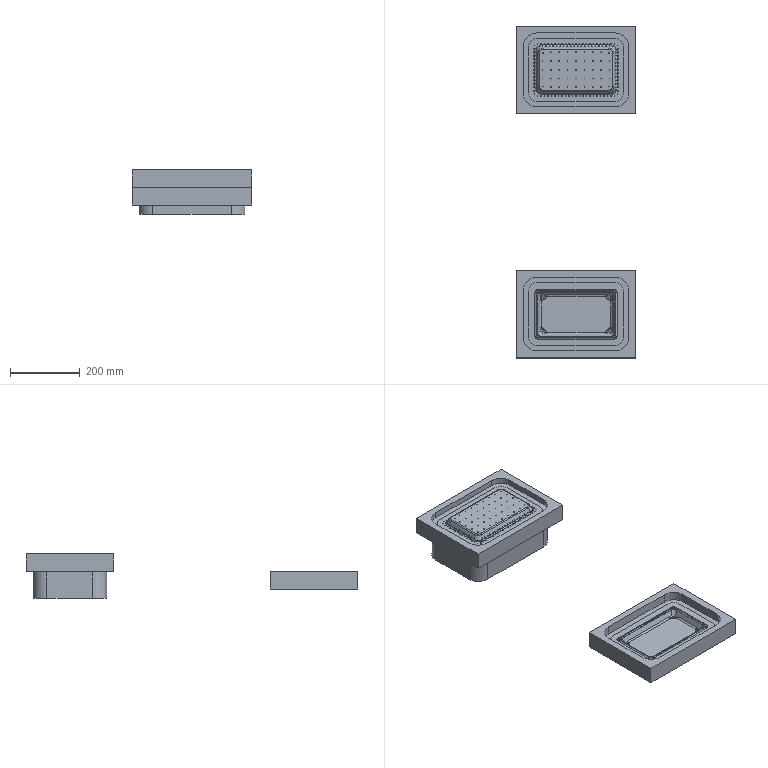NC program | NX | posted with a generic post | part box 343.99 x 952.259 x 127.368 mm
Lines 13167 to 13465 of 51088:
(FACE_MILLING_3 , TOOL : D10)
N26320 M6
N26322 G53
N26324 G17 G0 G90 X32.555 Y-435.842 S8000 M3 M8
N26326 G43 Z150. H0
N26328 Z-23.132
N26330 G94 G1 X30.696 Y-433.15 Z-23.304 F4000.
N26332 X29.631 Y-430.905 Z-23.434
N26334 X28.583 Y-428.447 Z-23.574
N26336 X28.334 Y-427.815 Z-23.61
N26338 X27.767 Y-426.062 Z-23.706
N26340 X27.14 Y-423.633 Z-23.838
N26342 X26.704 Y-421.216 Z-23.966
N26344 X26.456 Y-418.791 Z-24.094
N26346 X26.185 Y-411.39 Z-24.482
N26348 X26.075 Y-401.47 Z-25.002
N26350 X26.069 Y-398.988 Z-25.132
N26352 Y-287.228
N26354 X26.158 Y-282.314
N26356 X27.484 Y-274.956
N26358 X28.077 Y-273.223
N26360 X28.306 Y-272.553
N26362 X30.76 Y-267.71
N26364 X32.22 Y-265.229
N26366 X35.605 Y-261.599
N26368 X36.651 Y-260.556
N26370 X38.035 Y-259.307
N26372 X39.49 Y-258.132
N26374 X43.063 Y-255.634
N26376 X48.314 Y-253.023
N26378 X52.575 Y-252.129
N26380 X55.016 Y-251.677
N26382 X57.447 Y-251.445
N26384 X64.875 Y-251.175
N26386 X74.826 Y-251.062
N26388 X284.103 Y-251.073
N26390 X286.566 Y-251.245
N26392 X289.015 Y-251.41
N26394 X295.661 Y-253.019
N26396 X301.134 Y-255.762
N26398 G2 X309.666 Y-262.962 R40.7
N26400 G1 X310.985 Y-264.384
N26402 X311.762 Y-265.227
N26404 X313.409 Y-268.14
N26406 X314.35 Y-270.204
N26408 X315.4 Y-272.665
N26410 X315.664 Y-273.344
N26412 X316.219 Y-275.06
N26414 X316.91 Y-277.508
N26416 X317.577 Y-279.876
N26418 X317.929 Y-284.761
N26420 X317.914 Y-413.886
N26422 X317.877 Y-416.364
N26424 X317.841 Y-418.793
N26426 X317.356 Y-421.184
N26428 G2 X314.352 Y-430.907 R35.587
N26430 G1 X313.436 Y-432.893
N26432 X313.053 Y-433.612
N26434 X311.67 Y-435.876
N26436 X311.053 Y-436.873
N26438 X306.146 Y-442.057
N26440 X304.68 Y-443.186
N26442 X303.721 Y-443.924
N26444 X300.999 Y-445.498
N26446 X296.244 Y-447.59
N26448 G2 X286.546 Y-449.698 R36.192
N26450 G1 X279.123 Y-449.968
N26452 X269.172 Y-450.078
N26454 X62.373 Y-450.03
N26456 X59.882 Y-450.006
N26458 X57.427 Y-449.981
N26460 X54.987 Y-449.646
N26462 X52.539 Y-449.31
N26464 X47.753 Y-447.611
N26466 X43.014 Y-445.477
N26468 X39.466 Y-442.985
N26470 X38.035 Y-441.791
N26472 X36.619 Y-440.555
N26474 X35.615 Y-439.539
N26476 X34.372 Y-438.14
N26478 X33.176 Y-436.701
N26480 X30.696 Y-433.15
N26482 X29.631 Y-430.905
N26484 G2 X26.456 Y-418.791 R33.318
N26486 G1 X26.185 Y-411.39
N26488 X26.075 Y-401.47
N26490 X26.069 Y-398.988
N26492 X33.069 Y-398.979
N26494 Y-287.291
N26496 X33.146 Y-283.002
N26498 X34.278 Y-276.721
N26500 X34.775 Y-275.27
N26502 X36.942 Y-271.007
N26504 X37.872 Y-269.426
N26506 X40.629 Y-266.475
N26508 X41.47 Y-265.637
N26510 X42.582 Y-264.633
N26512 X43.726 Y-263.709
N26514 X44.503 Y-263.154
N26516 X46.564 Y-261.709
N26518 X48.412 Y-260.777
N26520 X50.607 Y-259.694
N26522 X51.517 Y-259.504
N26524 X53.931 Y-258.997
N26526 X55.988 Y-258.616
N26528 X57.928 Y-258.431
N26530 X65.051 Y-258.173
N26532 X74.848 Y-258.062
N26534 X283.859 Y-258.073
N26536 X286.087 Y-258.228
N26538 X287.948 Y-258.354
N26540 X293.272 Y-259.643
N26542 X295.588 Y-260.785
N26544 X297.445 Y-261.722
N26546 G2 X304.543 Y-267.731 R33.421
N26548 G1 X306.088 Y-269.4
N26550 X307.04 Y-271.046
N26552 X307.946 Y-273.03
N26554 X308.917 Y-275.309
N26556 X309.067 Y-275.692
N26558 X309.518 Y-277.088
N26560 X310.173 Y-279.408
N26562 X310.646 Y-281.089
N26564 X310.93 Y-285.018
N26566 X310.914 Y-413.832
N26568 X310.851 Y-418.039
N26570 X310.495 Y-419.793
N26572 G2 X307.959 Y-428.052 R29.313
N26574 G1 X307.079 Y-429.963
N26576 X305.47 Y-432.593
N26578 X301.452 Y-436.837
N26580 X299.806 Y-438.104
N26582 X297.895 Y-439.219
N26584 X293.396 Y-441.176
N26586 X291.92 Y-441.643
N26588 X289.918 Y-442.157
N26590 X287.987 Y-442.503
N26592 X286.024 Y-442.714
N26594 X278.947 Y-442.97
N26596 X269.15 Y-443.078
N26598 X62.442 Y-443.031
N26600 X59.952 Y-443.006
N26602 X57.94 Y-442.986
N26604 X54.168 Y-442.468
N26606 X50.454 Y-441.152
N26608 X48.174 Y-440.152
N26610 X46.444 Y-439.351
N26612 G2 X40.724 Y-434.75 R33.121
N26614 G1 X39.683 Y-433.578
N26616 X38.711 Y-432.409
N26618 X38.179 Y-431.672
N26620 X36.816 Y-429.718
N26622 X36.015 Y-428.031
N26624 G2 X33.441 Y-418.286 R26.439
N26626 G1 X33.183 Y-411.213
N26628 X33.075 Y-401.449
N26630 X33.069 Y-398.979
N26632 X40.069 Y-398.97
N26634 Y-287.354
N26636 X40.135 Y-283.689
N26638 X41.073 Y-278.487
N26640 X41.244 Y-277.987
N26642 X42.976 Y-274.557
N26644 X43.521 Y-273.629
N26646 X46.288 Y-270.717
N26648 X47.128 Y-269.959
N26650 X47.961 Y-269.286
N26652 X48.547 Y-268.868
N26654 X50.168 Y-267.731
N26656 X51.536 Y-267.042
N26658 X52.91 Y-266.364
N26660 X56.959 Y-265.555
N26662 X58.408 Y-265.417
N26664 X65.227 Y-265.171
N26666 X74.869 Y-265.062
N26668 X283.615 Y-265.073
N26670 X285.608 Y-265.212
N26672 X286.882 Y-265.298
N26674 X290.87 Y-266.263
N26676 X293.861 Y-267.754
N26678 X295.432 Y-268.841
N26680 X295.909 Y-269.189
N26682 X296.871 Y-269.984
N26684 X297.771 Y-270.778
N26686 X300.419 Y-273.579
N26688 X300.812 Y-274.258
N26690 X302.469 Y-278.041
N26692 X303.436 Y-281.308
N26694 X303.716 Y-282.302
N26696 X303.93 Y-285.275
N26698 X303.914 Y-413.779
N26700 X303.862 Y-417.284
N26702 X303.635 Y-418.401
N26704 X303.214 Y-420.48
N26706 X302.791 Y-422.117
N26708 X302.318 Y-423.461
N26710 X301.567 Y-425.198
N26712 X300.892 Y-426.663
N26714 X299.881 Y-428.319
N26716 X296.758 Y-431.617
N26718 X295.891 Y-432.284
N26720 X294.685 Y-432.988
N26722 X293.067 Y-433.717
N26724 G2 X285.501 Y-435.729 R20.713
N26726 G1 X278.772 Y-435.973
N26728 X269.129 Y-436.078
N26730 X62.512 Y-436.031
N26732 X60.022 Y-436.006
N26734 X58.453 Y-435.99
N26736 X55.797 Y-435.626
N26738 X52.997 Y-434.624
N26740 X51.05 Y-433.77
N26742 X49.953 Y-433.262
N26744 G2 X45.833 Y-429.962 R24.933
N26746 G1 X44.993 Y-429.016
N26748 X44.246 Y-428.117
N26750 X43.887 Y-427.619
N26752 X42.891 Y-426.191
N26754 X41.539 Y-423.137
N26756 X41.217 Y-422.153
N26758 X40.825 Y-420.636
N26760 X40.577 Y-419.26
N26762 X40.426 Y-417.781
N26764 X40.18 Y-411.037
N26766 X40.075 Y-401.428
N26768 X40.069 Y-398.97
N26770 X47.069 Y-398.961
N26772 Y-287.417
N26774 X47.124 Y-284.376
N26776 X47.827 Y-280.477
N26778 X49.166 Y-277.84
N26780 X51.107 Y-275.797
N26782 X51.675 Y-275.285
N26784 X52.197 Y-274.863
N26786 X52.591 Y-274.582
N26788 X53.773 Y-273.753
N26790 X54.66 Y-273.306
N26792 X55.183 Y-273.048
N26794 X57.979 Y-272.49
N26796 X58.888 Y-272.403
N26798 X65.403 Y-272.169
N26800 X74.891 Y-272.062
N26802 X283.371 Y-272.073
N26804 X285.128 Y-272.195
N26806 X285.815 Y-272.242
N26808 X286.481 Y-272.403
N26810 X288.469 Y-272.884
N26812 X289.338 Y-273.313
N26814 X290.277 Y-273.786
N26816 G2 X294.682 Y-277.688 R18.575
N26818 G1 X295.136 Y-278.683
N26820 X295.896 Y-280.463
N26822 X296.785 Y-283.515
N26824 X296.93 Y-285.533
N26826 X296.914 Y-413.726
N26828 X296.872 Y-416.529
N26830 X296.775 Y-417.01
N26832 X296.39 Y-418.908
N26834 X296.07 Y-420.146
N26836 X295.894 Y-420.682
N26838 X295.175 Y-422.343
N26840 X294.705 Y-423.363
N26842 X294.285 Y-424.05
N26844 X291.976 Y-426.464
N26846 X291.475 Y-426.756
N26848 X290.247 Y-427.31
N26850 G2 X284.979 Y-428.745 R13.919
N26852 G1 X278.596 Y-428.975
N26854 X269.107 Y-429.078
N26856 X62.581 Y-429.031
N26858 X60.092 Y-429.007
N26860 X58.967 Y-428.995
N26862 X57.425 Y-428.784
N26864 X57.093 Y-428.669
N26866 X55.81 Y-428.214
N26868 X53.927 Y-427.388
N26870 X53.463 Y-427.173
N26872 G2 X48.965 Y-422.665 R14.8
N26874 X47.411 Y-417.276 R13.226
N26876 G1 X47.178 Y-410.861
N26878 X47.075 Y-401.407
N26880 X47.069 Y-398.961
N26882 X49.456
N26884 Y-287.275
N26886 G2 X62.275 Y-274.456 R12.819
N26888 G1 X281.715
N26890 G2 X294.534 Y-287.275 R12.819
N26892 G1 Y-413.854
N26894 G2 X281.715 Y-426.673 R12.819
N26896 G1 X62.275
N26898 G2 X49.456 Y-413.854 R12.819
N26900 G1 Y-398.961
N26902 G3 X47.456 Y-396.961 R2.
N26904 G1 Z-24.132
N26906 G0 Z150.
N26908 M9
N26910 M5